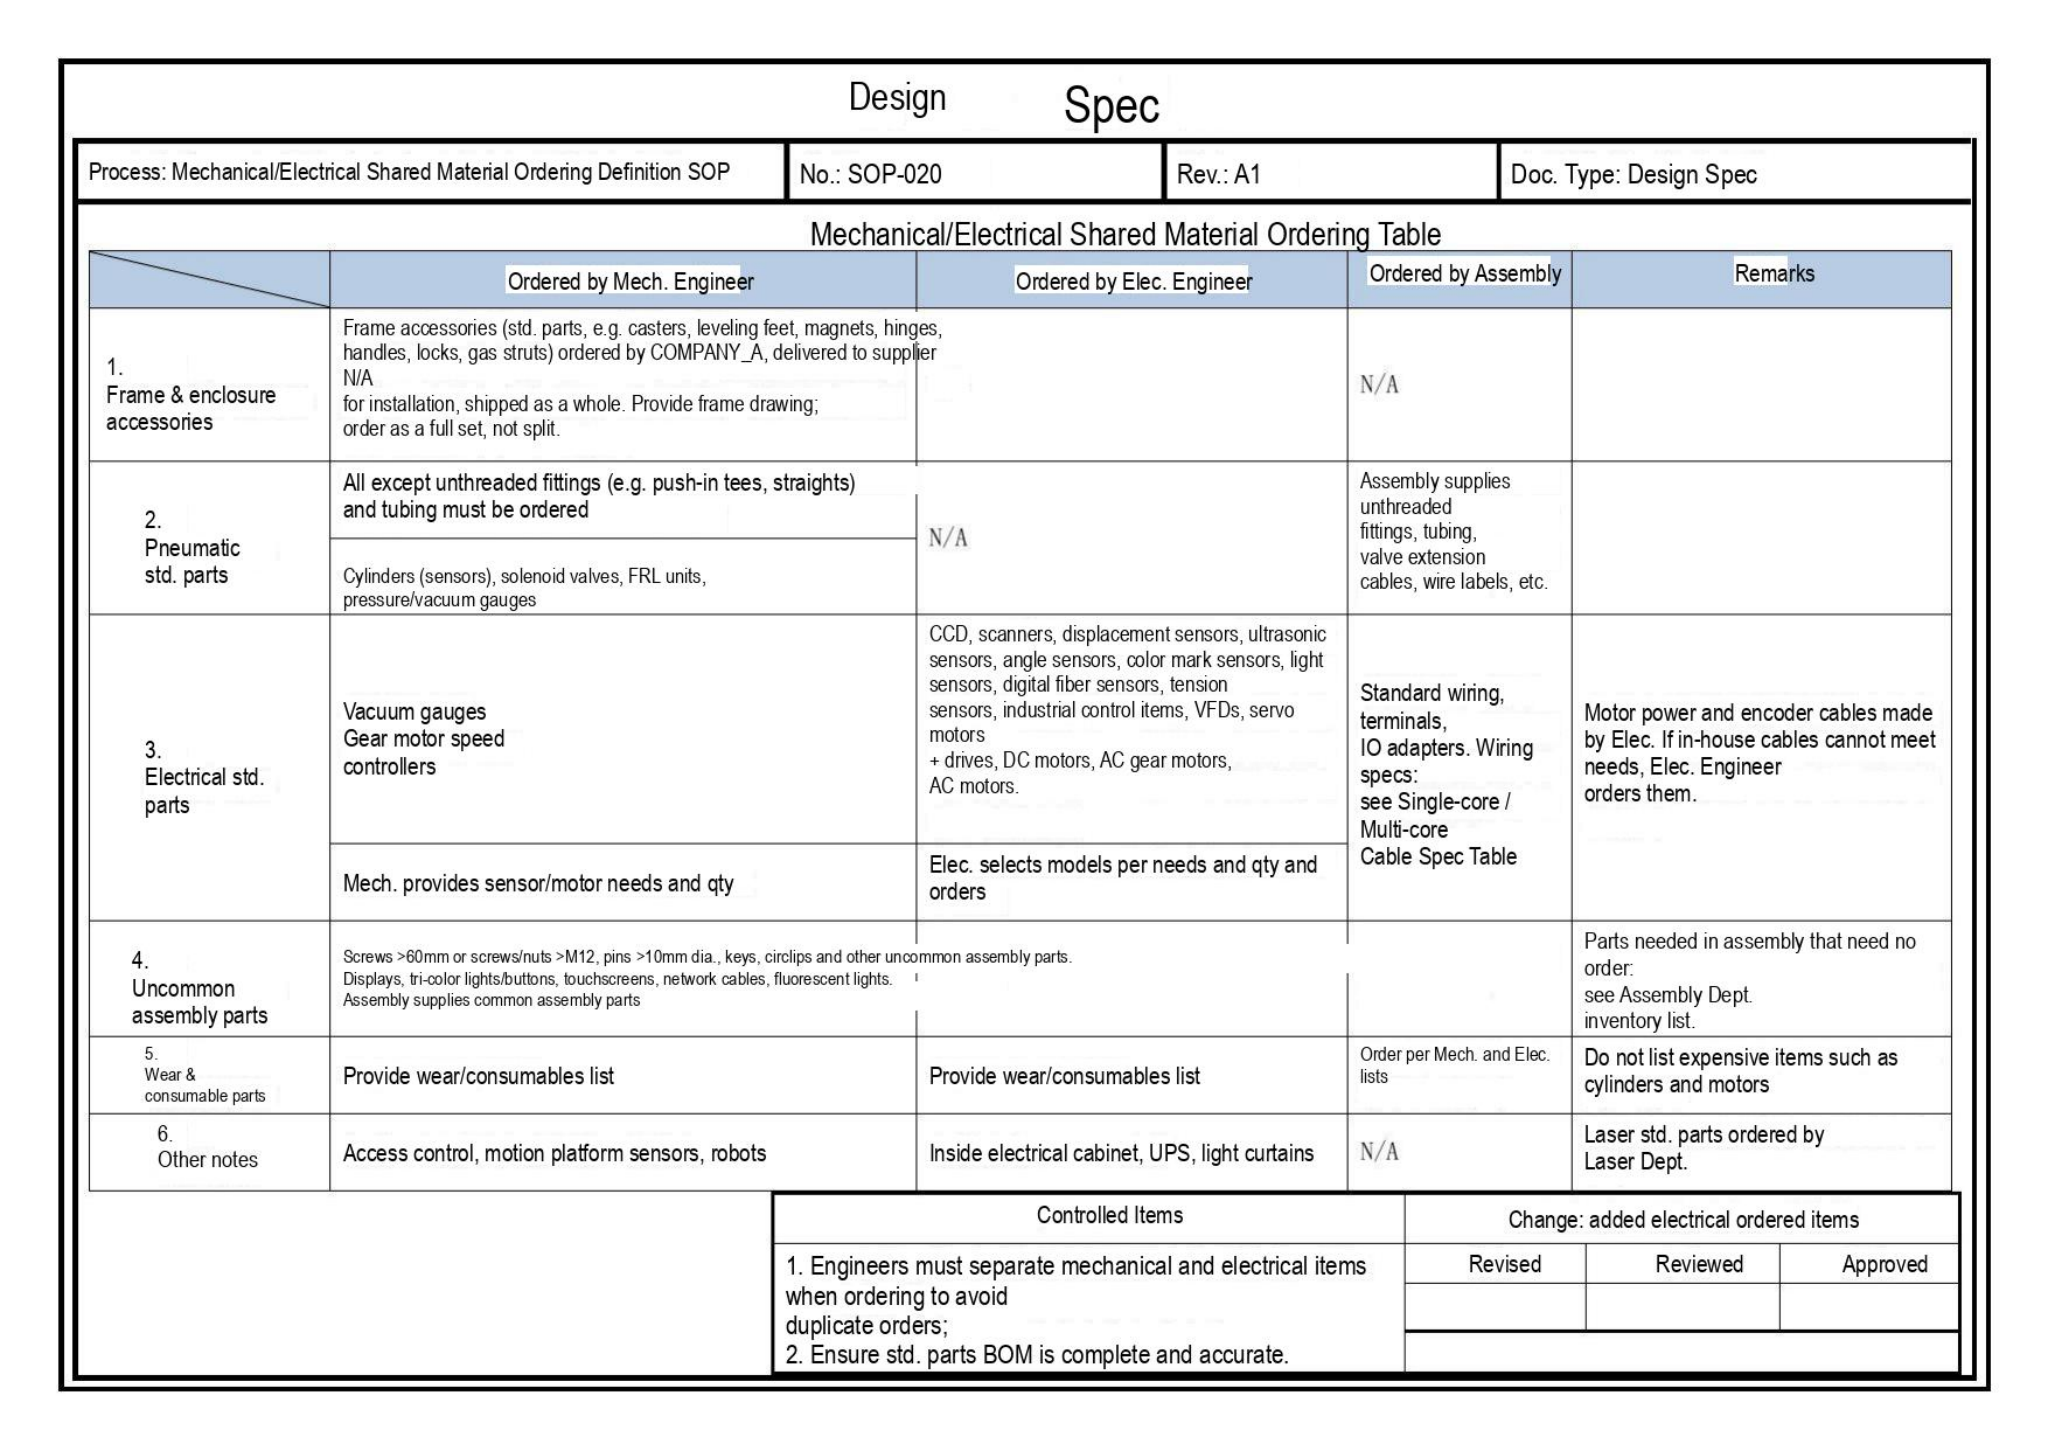Design Spec

| Process: Mechanical/Electrical Shared Material Ordering Definition SOP | No.: SOP-020 | Rev.: A1 | Doc. Type: Design Spec |
|---|---|---|---|

Mechanical/Electrical Shared Material Ordering Table

| | Ordered by Mech. Engineer | Ordered by Elec. Engineer | Ordered by Assembly | Remarks |
|---|---|---|---|---|
| 1. Frame & enclosure accessories | Frame accessories (std. parts, e.g. casters, leveling feet, magnets, hinges, handles, locks, gas struts) ordered by COMPANY_A, delivered to supplier N/A for installation, shipped as a whole. Provide frame drawing; order as a full set, not split. | | N/A | |
| 2. Pneumatic std. parts | All except unthreaded fittings (e.g. push-in tees, straights) and tubing must be ordered | N/A | Assembly supplies unthreaded fittings, tubing, valve extension cables, wire labels, etc. | |
| | Cylinders (sensors), solenoid valves, FRL units, pressure/vacuum gauges | | | |
| 3. Electrical std. parts | Vacuum gauges Gear motor speed controllers | CCD, scanners, displacement sensors, ultrasonic sensors, angle sensors, color mark sensors, light sensors, digital fiber sensors, tension sensors, industrial control items, VFDs, servo motors + drives, DC motors, AC gear motors, AC motors. | Standard wiring, terminals, IO adapters. Wiring specs: see Single-core / Multi-core Cable Spec Table | Motor power and encoder cables made by Elec. If in-house cables cannot meet needs, Elec. Engineer orders them. |
| | Mech. provides sensor/motor needs and qty | Elec. selects models per needs and qty and orders | | |
| 4. Uncommon assembly parts | Screws >60mm or screws/nuts >M12, pins >10mm dia., keys, circlips and other uncommon assembly parts. Displays, tri-color lights/buttons, touchscreens, network cables, fluorescent lights. Assembly supplies common assembly parts | | | Parts needed in assembly that need no order: see Assembly Dept. inventory list. |
| 5. Wear & consumable parts | Provide wear/consumables list | Provide wear/consumables list | Order per Mech. and Elec. lists | Do not list expensive items such as cylinders and motors |
| 6. Other notes | Access control, motion platform sensors, robots | Inside electrical cabinet, UPS, light curtains | N/A | Laser std. parts ordered by Laser Dept. |

| Controlled Items | Change: added electrical ordered items | | |
|---|---|---|---|
| 1. Engineers must separate mechanical and electrical items when ordering to avoid duplicate orders; 2. Ensure std. parts BOM is complete and accurate. | Revised | Reviewed | Approved |
| | | | |